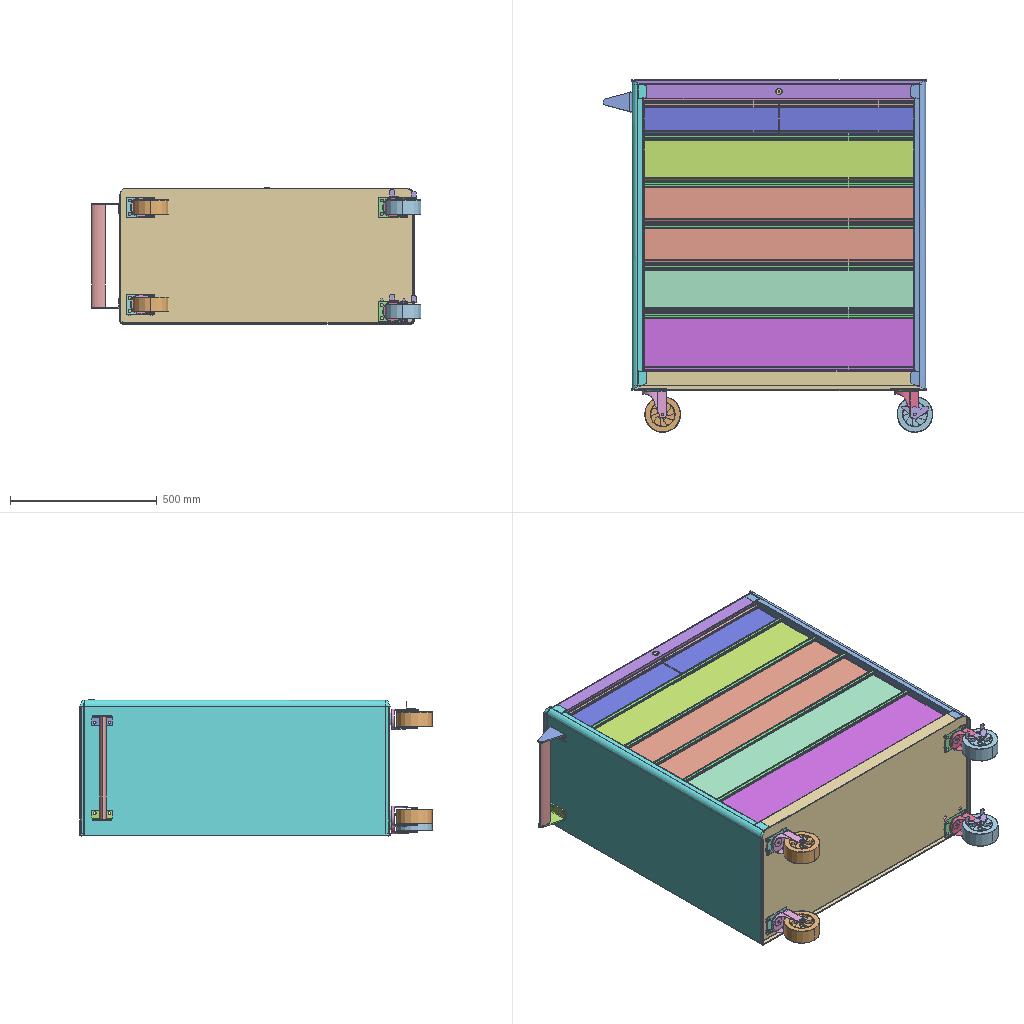Assembly | SolidWorks | 19 different items | 28 placed | box 1122 x 1201 x 465 mm
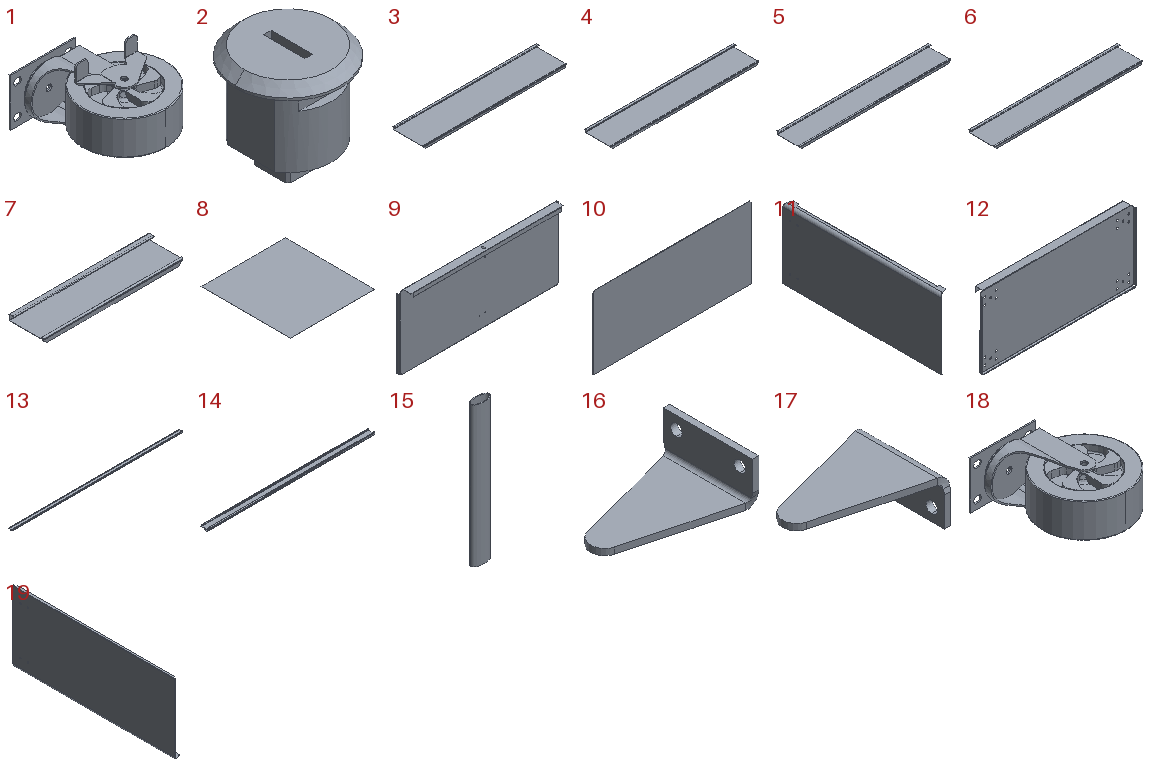Parts list (item | quantity | size | volume | features):
1 | x2 | 143 x 148.5 x 94.5 mm | 569574 mm3 | features BaseBody 10, CombineBodies 2
2 | x1 | 23 x 23 x 22.5 mm | 4876 mm3 | features BaseBody 1
3 | x1 | 915 x 196.571 x 33.2 mm | 189594 mm3 | features SM3dBend 4, EdgeFlange 2, FlatPattern 1, Hem 1, SMBaseFlange 1, SheetMetal 1
4 | x1 | 915 x 160.571 x 33.2 mm | 163242 mm3 | features SM3dBend 4, EdgeFlange 2, FlatPattern 1, Hem 1, SMBaseFlange 1, SheetMetal 1
5 | x2 | 915 x 136.571 x 33.2 mm | 145674 mm3 | features SM3dBend 4, EdgeFlange 2, FlatPattern 1, Hem 1, SMBaseFlange 1, SheetMetal 1
6 | x1 | 915 x 157.414 x 33.2 mm | 160931 mm3 | features SM3dBend 4, EdgeFlange 2, FlatPattern 1, Hem 1, SMBaseFlange 1, SheetMetal 1
7 | x2 | 455 x 111.371 x 33.2 mm | 63198 mm3 | features SM3dBend 4, EdgeFlange 2, FlatPattern 1, Hem 1, SMBaseFlange 1, SheetMetal 1
8 | x1 | 998.4 x 1055 x 0.8 mm | 842809 mm3 | features FlatPattern 1, SMBaseFlange 1, SheetMetal 1
9 | x1 | 1007 x 66.2 x 462.807 mm | 677341 mm3 | features EdgeFlange 7, ICE 5, RevCut 2, Revolution 2, FlatPattern 1, SM3dBend 1, SMBaseFlange 1, SheetMetal 1
10 | x1 | 994.2 x 2.032 x 454.9 mm | 918733 mm3 | features FlatPattern 1, SMBaseFlange 1, SheetMetal 1
11 | x1 | 50 x 1055 x 460.8 mm | 442365 mm3 | features EdgeFlange 3, FlatPattern 1, HoleWzd 1, SMBaseFlange 1, SheetMetal 1
12 | x1 | 1007 x 66.2 x 462.805 mm | 687365 mm3 | features ICE 18, EdgeFlange 8, FlatPattern 1, HoleWzd 1, SMBaseFlange 1, SheetMetal 1
13 | x5 | 915 x 19.991 x 9 mm | 36941 mm3 | features Extrusion 1
14 | x2 | 455 x 19.991 x 9 mm | 18370 mm3 | features Extrusion 1
15 | x1 | 47.25 x 22 x 348 mm | 56835 mm3 | features Extrusion 1
16 | x1 | 97.999 x 70.526 x 35.001 mm | 30038 mm3 | features Fillet 2, BaseBody 1, HoleWzd 1, ICE 1
17 | x1 | 97.999 x 70.526 x 35.001 mm | 30038 mm3 | features Fillet 2, BaseBody 1, HoleWzd 1, ICE 1
18 | x2 | 143 x 148.5 x 70 mm | 563559 mm3 | features BaseBody 10, CombineBodies 2
19 | x1 | 50 x 1055 x 460.8 mm | 442365 mm3 | features MirrorStock 1
Mates (type | each side: item.copy, entity, surface, feature):
Coincident | 8.1 face plane Base-Flange1 | 11.1 face plane Edge-Flange1
Coincident | 8.1 face plane Base-Flange1 | 11.1 face plane Base-Flange1
Coincident | 11.1 face plane Edge-Flange2 | 9.1 face plane Sketched Bend1 | 2 times
Coincident | 12.1 face plane Edge-Flange1 | 11.1 face plane Edge-Flange2
Coincident | 11.1 face plane Edge-Flange3 | 12.1 face plane Edge-Flange5
Coincident | 16.1 edge | 11.1 edge | 2 times
Coincident | 15.1 face plane Boss-Extrude1 | 17.1 face plane Imported3
Concentric | 1.1 edge | 12.1 edge
DistanceDim | 18.1 face plane Imported42 | 12.1 face plane Base-Flange1
Concentric | 18.1 edge | 12.1 edge
Coincident | 10.1 face plane Base-Flange1 | 9.1 face plane Base-Flange1
Coincident | 10.1 face plane Base-Flange1 | 9.1 face plane Edge-Flange2
Coincident | 3.1 face plane Hem1 | 13.1 edge
Coincident | 3.1 face plane Edge-Flange2 | 13.1 face plane Boss-Extrude1 | 2 times
Coincident | 3.1 face plane Base-Flange1 | 4.1 face plane Base-Flange1
Coincident | 3.1 face plane Edge-Flange1 | 4.1 face plane Edge-Flange1
Coincident | 13.1 face plane Boss-Extrude1 | 13.2 face plane Boss-Extrude1
Coincident | 4.1 face plane Edge-Flange2 | 13.2 edge
Coincident | 4.1 face plane Edge-Flange1 | 5.1 face plane Edge-Flange1
Coincident | 4.1 face plane Base-Flange1 | 5.1 face plane Base-Flange1
Coincident | 13.2 face plane Boss-Extrude1 | 13.3 face plane Boss-Extrude1 | 2 times
Coincident | 5.1 face plane Base-Flange1 | 5.2 face plane Base-Flange1 | 2 times
Coincident | 5.1 face plane Edge-Bend2 | 5.2 face plane Edge-Flange1
Coincident | 13.4 face plane Boss-Extrude1 | 13.3 face plane Boss-Extrude1
Coincident | 13.4 face plane Boss-Extrude1 | 5.2 face plane Edge-Flange1
Coincident | 7.1 face plane Base-Flange1 | 7.2 face plane Base-Flange1
Coincident | 7.1 face plane Edge-Flange1 | 7.2 face plane Edge-Flange1 | 2 times
Coincident | 13.4 face plane Boss-Extrude1 | 13.5 face plane Boss-Extrude1
Coincident | 13.5 face plane Boss-Extrude1 | 14.1 face plane Boss-Extrude1
Coincident | 7.1 face plane Edge-Flange2 | 14.1 face plane Boss-Extrude1
Coincident | 14.1 face plane Boss-Extrude1 | 14.2 face plane Boss-Extrude1 | 2 times
Coincident | 7.2 face plane Edge-Flange1 | 14.2 face plane Boss-Extrude1
Coincident | 8.1 face plane Base-Flange1 | assembly plane
Concentric | 2.1 face cylinder Lock | 9.1 face cylinder Cut-Extrude5
Coincident | 2.1 face plane Lock | 9.1 face plane Sketched Bend1
DistanceDim | 3.1 edge | 12.1 face plane Edge-Flange5
DistanceDim | 3.1 face plane Edge-Flange1 | 4.1 face cylinder Sketch Bend3
DistanceDim | 4.1 face plane Edge-Flange1 | 5.1 face cylinder Sketch Bend3
DistanceDim | 5.1 face plane Edge-Flange1 | 5.2 face cylinder Sketch Bend3
Tangent | 9.1 face cylinder Edge-Bend7 | assembly plane
Width | 10.1 face plane Base-Flange1 | 10.1 face plane Base-Flange1 | 19.1 face plane Side Plate1_Mirror1 | 11.1 face plane Base-Flange1
Width | 9.1 face plane Edge-Flange1 | 9.1 face plane Edge-Flange3 | 19.1 face plane Side Plate1_Mirror1 | 11.1 face plane Base-Flange1
Width | 12.1 face plane Edge-Flange2 | 12.1 face plane Edge-Flange4 | 19.1 face plane Side Plate1_Mirror1 | 11.1 face plane Base-Flange1
DistanceDim | 19.1 face plane Side Plate1_Mirror1 | 12.1 face plane Edge-Flange4
DistanceDim | 1.1 face plane Imported38 | 12.1 face plane Base-Flange1
Parallel | 1.1 face plane Imported51 | 12.1 face plane Edge-Flange1
Parallel | 18.1 face plane Imported16 | 12.1 face plane Edge-Flange1
Parallel | 8.1 plane | 9.1 face plane Edge-Flange1
Width | 8.1 face plane Base-Flange1 | 8.1 face plane Base-Flange1 | 19.1 face plane Side Plate1_Mirror1 | 11.1 face plane Base-Flange1
Width | 3.1 face plane Base-Flange1 | 3.1 face plane Edge-Flange1 | 19.1 face plane Side Plate1_Mirror1 | 11.1 face plane Base-Flange1
DistanceDim | 3.1 face plane Base-Flange1 | 19.1 face plane Side Plate1_Mirror1
Coincident | 11.1 edge | 9.1 face cylinder Edge-Bend5
Parallel | 11.1 face plane Base-Flange1 | assembly plane
Coincident | 11.1 face plane Base-Flange1 | assembly select_type:10
DistanceDim | 13.2 face plane Boss-Extrude1 | 4.1 face plane Edge-Flange1
DistanceDim | 13.3 face plane Boss-Extrude1 | 5.1 face plane Edge-Flange1
DistanceDim | 13.4 face plane Boss-Extrude1 | 5.2 face plane Edge-Flange1
Parallel | 15.1 plane | 10.1 face plane Base-Flange1
Tangent | 15.1 face surface:4009 Boss-Extrude1 | 17.1 edge
DistanceDim | 6.1 face plane Sketched Bend1 | 5.2 face plane Edge-Flange1
Coincident | 7.2 face plane Edge-Flange1 | 6.1 face plane Edge-Flange2
Coincident | 5.2 face plane Base-Flange1 | 6.1 face plane Base-Flange1
DistanceDim | 13.5 face plane Boss-Extrude1 | 6.1 face plane Edge-Flange1
Coincident | 13.5 face plane Boss-Extrude1 | 6.1 face plane Edge-Flange1
Coincident | 7.1 face plane Base-Flange1 | 6.1 face plane Base-Flange1
Coincident | 7.1 face plane Edge-Flange1 | 6.1 face plane Edge-Flange1
Coincident | 7.2 face plane Edge-Flange1 | 6.1 face plane Edge-Flange1